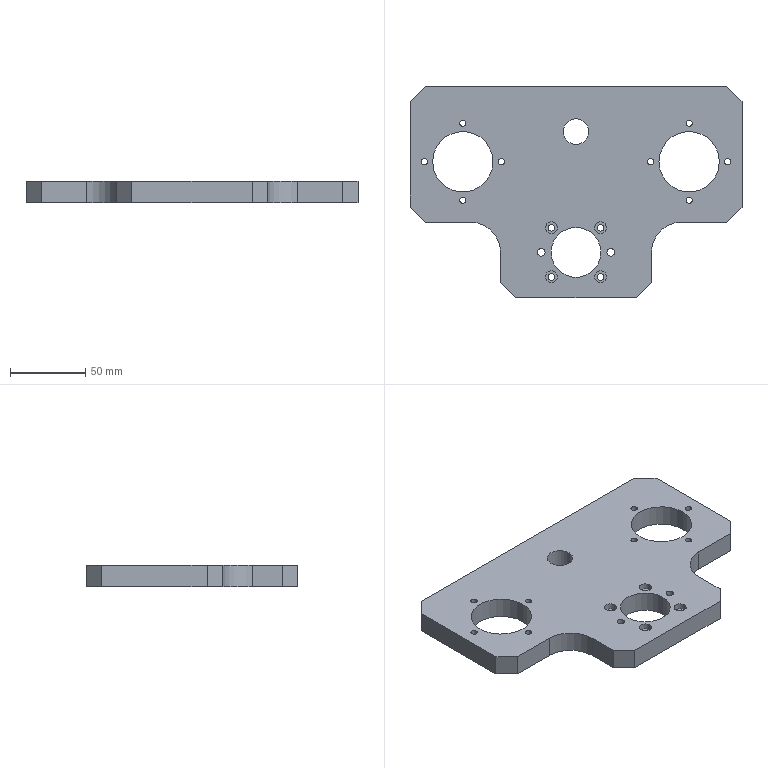Part | STEP file | fBY02F02M-00-07A | 1 solid | 66 faces | box 220 x 140 x 14 mm | volume 291524 mm3 | cylinder 46 | plane 20 | commonest cylinder face diameters 4.2 x16 4.5 x8 8 x8 40 x6 5 x4 17 x2